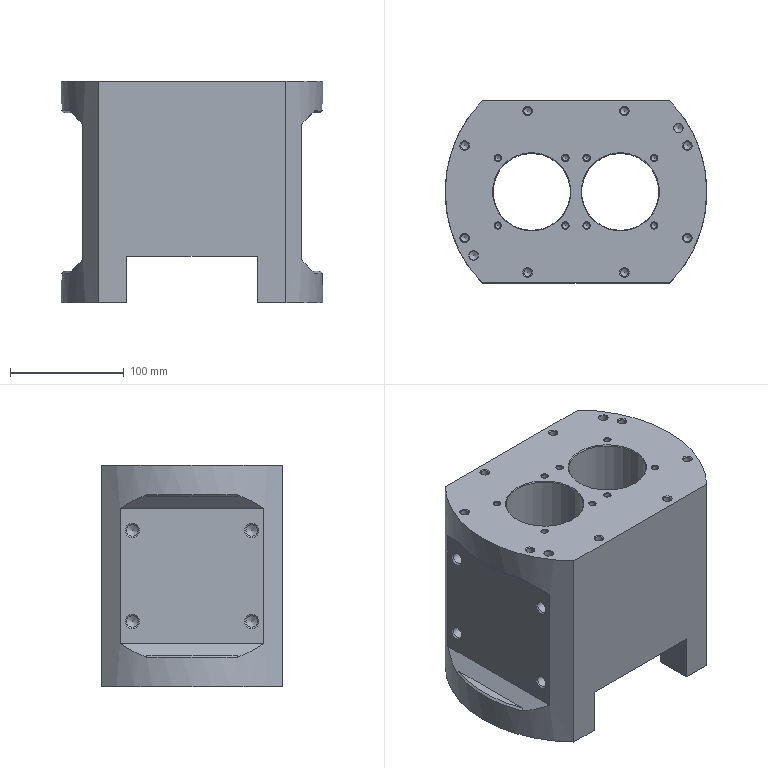NC program | NX | posted with a generic post | part box 230 x 160 x 195 mm
Whole program:
N10 G17 G21 G94 G90
(FLOOR_WALL_COPY_1 , TOOL : D50)
N12 T02 M6
N14 G54
N16 G17 G0 G90 X46.956 Y-107.497 B0. C0. S1200 M3
N18 G43 Z30. H2
N20 Z2.651
N22 G94 G1 Z-0.349 F1000.
N24 X43.956
N26 X-43.956 F2000.
N28 Y-68.498
N30 X43.956
N32 Y-29.498
N34 X-43.956
N36 Y9.501
N38 X43.956
N40 Y48.501
N42 X-43.956
N44 Y87.5
N46 X43.956
N48 X46.956
N50 Z2.651
N52 G0 Z30.
N54 X50.654 Y-107.497
N56 Z2.302
N58 G1 Z-0.698 F1000.
N60 X47.654
N62 X-47.654 F2000.
N64 Y-68.498
N66 X47.654
N68 Y-29.498
N70 X-47.654
N72 Y9.501
N74 X47.654
N76 Y48.501
N78 X-47.654
N80 Y87.5
N82 X47.654
N84 X50.654
N86 Z2.302
N88 G0 Z30.
N90 X53.485 Y-107.497
N92 Z1.953
N94 G1 Z-1.047 F1000.
N96 X50.485
N98 X-50.485 F2000.
N100 Y-68.498
N102 X50.485
N104 Y-29.498
N106 X-50.485
N108 Y9.501
N110 X50.485
N112 Y48.501
N114 X-50.485
N116 Y87.5
N118 X50.485
N120 X53.485
N122 Z1.953
N124 G0 Z30.
N126 X55.866 Y-107.497
N128 Z1.604
N130 G1 Z-1.396 F1000.
N132 X52.866
N134 X-52.866 F2000.
N136 Y-68.498
N138 X52.866
N140 Y-29.498
N142 X-52.866
N144 Y9.501
N146 X52.866
N148 Y48.501
N150 X-52.866
N152 Y87.5
N154 X52.866
N156 X55.866
N158 Z1.604
N160 G0 Z30.
N162 X57.959 Y-107.497
N164 Z1.255
N166 G1 Z-1.745 F1000.
N168 X54.959
N170 X-54.959 F2000.
N172 Y-68.498
N174 X54.959
N176 Y-29.498
N178 X-54.959
N180 Y9.501
N182 X54.959
N184 Y48.501
N186 X-54.959
N188 Y87.5
N190 X54.959
N192 X57.959
N194 Z1.255
N196 G0 Z30.
N198 X59.847 Y-107.497
N200 Z0.906
N202 G1 Z-2.094 F1000.
N204 X56.847
N206 X-56.847 F2000.
N208 Y-68.498
N210 X56.847
N212 Y-29.498
N214 X-56.847
N216 Y9.501
N218 X56.847
N220 Y48.501
N222 X-56.847
N224 Y87.5
N226 X56.847
N228 X59.847
N230 Z0.906
N232 G0 Z30.
N234 X61.579 Y-107.497
N236 Z0.557
N238 G1 Z-2.443 F1000.
N240 X58.579
N242 X-58.579 F2000.
N244 Y-68.498
N246 X58.579
N248 Y-29.498
N250 X-58.579
N252 Y9.501
N254 X58.579
N256 Y48.501
N258 X-58.579
N260 Y87.5
N262 X58.579
N264 X61.579
N266 Z0.557
N268 G0 Z30.
N270 X63.188 Y-107.497
N272 Z0.208
N274 G1 Z-2.792 F1000.
N276 X60.188
N278 X-60.188 F2000.
N280 Y-68.498
N282 X60.188
N284 Y-29.498
N286 X-60.188
N288 Y9.501
N290 X60.188
N292 Y48.501
N294 X-60.188
N296 Y87.5
N298 X60.188
N300 X63.188
N302 Z0.208
N304 G0 Z30.
N306 X64.695 Y-107.497
N308 Z-0.141
N310 G1 Z-3.141 F1000.
N312 X61.695
N314 X-61.695 F2000.
N316 Y-68.498
N318 X61.695
N320 Y-29.498
N322 X-61.695
N324 Y9.501
N326 X61.695
N328 Y48.501
N330 X-61.695
N332 Y87.5
N334 X61.695
N336 X64.695
N338 Z-0.141
N340 G0 Z30.
N342 X66.117 Y-107.497
N344 Z-0.49
N346 G1 Z-3.49 F1000.
N348 X63.117
N350 X-63.117 F2000.
N352 Y-68.498
N354 X63.117
N356 Y-29.498
N358 X-63.117
N360 Y9.501
N362 X63.117
N364 Y48.501
N366 X-63.117
N368 Y87.5
N370 X63.117
N372 X66.117
N374 Z-0.49
N376 G0 Z30.
N378 X67.467 Y-107.497
N380 Z-0.839
N382 G1 Z-3.839 F1000.
N384 X64.467
N386 X-64.467 F2000.
N388 Y-68.498
N390 X64.467
N392 Y-29.498
N394 X-64.467
N396 Y9.501
N398 X64.467
N400 Y48.501
N402 X-64.467
N404 Y87.5
N406 X64.467
N408 X67.467
N410 Z-0.839
N412 G0 Z30.
N414 X68.753 Y-107.497
N416 Z-1.188
N418 G1 Z-4.188 F1000.
N420 X65.753
N422 X-65.753 F2000.
N424 Y-68.498
N426 X65.753
N428 Y-29.498
N430 X-65.753
N432 Y9.501
N434 X65.753
N436 Y48.501
N438 X-65.753
N440 Y87.5
N442 X65.753
N444 X68.753
N446 Z-1.188
N448 G0 Z30.
N450 X69.984 Y-107.497
N452 Z-1.537
N454 G1 Z-4.537 F1000.
N456 X66.984
N458 X-66.984 F2000.
N460 Y-68.498
N462 X66.984
N464 Y-29.498
N466 X-66.984
N468 Y9.501
N470 X66.984
N472 Y48.501
N474 X-66.984
N476 Y87.5
N478 X66.984
N480 X69.984
N482 Z-1.537
N484 G0 Z30.
N486 X71.166 Y-107.497
N488 Z-1.886
N490 G1 Z-4.886 F1000.
N492 X68.166
N494 X-68.166 F2000.
N496 Y-68.498
N498 X68.166
N500 Y-29.498
N502 X-68.166
N504 Y9.501
N506 X68.166
N508 Y48.501
N510 X-68.166
N512 Y87.5
N514 X68.166
N516 X71.166
N518 Z-1.886
N520 G0 Z30.
N522 X72.303 Y-107.497
N524 Z-2.235
N526 G1 Z-5.235 F1000.
N528 X69.303
N530 X-69.303 F2000.
N532 Y-68.498
N534 X69.303
N536 Y-29.498
N538 X-69.303
N540 Y9.501
N542 X69.303
N544 Y48.501
N546 X-69.303
N548 Y87.5
N550 X69.303
N552 X72.303
N554 Z-2.235
N556 G0 Z30.
N558 X73.4 Y-107.497
N560 Z-2.584
N562 G1 Z-5.584 F1000.
N564 X70.4
N566 X-70.4 F2000.
N568 Y-68.498
N570 X70.4
N572 Y-29.498
N574 X-70.4
N576 Y9.501
N578 X70.4
N580 Y48.501
N582 X-70.4
N584 Y87.5
N586 X70.4
N588 X73.4
N590 Z-2.584
N592 G0 Z30.
N594 X74.462 Y-107.497
N596 Z-2.933
N598 G1 Z-5.933 F1000.
N600 X71.462
N602 X-71.462 F2000.
N604 Y-68.498
N606 X71.462
N608 Y-29.498
N610 X-71.462
N612 Y9.501
N614 X71.462
N616 Y48.501
N618 X-71.462
N620 Y87.5
N622 X71.462
N624 X74.462
N626 Z-2.933
N628 G0 Z30.
N630 X75.489 Y-107.497
N632 Z-3.282
N634 G1 Z-6.282 F1000.
N636 X72.489
N638 X-72.489 F2000.
N640 Y-68.498
N642 X72.489
N644 Y-29.498
N646 X-72.489
N648 Y9.501
N650 X72.489
N652 Y48.501
N654 X-72.489
N656 Y87.5
N658 X72.489
N660 X75.489
N662 Z-3.282
N664 G0 Z30.
N666 X76.487 Y-107.497
N668 Z-3.631
N670 G1 Z-6.631 F1000.
N672 X73.487
N674 X-73.487 F2000.
N676 Y-68.498
N678 X73.487
N680 Y-29.498
N682 X-73.487
N684 Y9.501
N686 X73.487
N688 Y48.501
N690 X-73.487
N692 Y87.5
N694 X73.487
N696 X76.487
N698 Z-3.631
N700 G0 Z30.
N702 X77.455 Y-107.497
N704 Z-3.98
N706 G1 Z-6.98 F1000.
N708 X74.455
N710 X-74.455 F2000.
N712 Y-68.498
N714 X74.455
N716 Y-29.498
N718 X-74.455
N720 Y9.501
N722 X74.455
N724 Y48.501
N726 X-74.455
N728 Y87.5
N730 X74.455
N732 X77.455
N734 Z-3.98
N736 G0 Z30.
N738 X78.398 Y-107.497
N740 Z-4.329
N742 G1 Z-7.329 F1000.
N744 X75.398
N746 X-75.398 F2000.
N748 Y-68.498
N750 X75.398
N752 Y-29.498
N754 X-75.398
N756 Y9.501
N758 X75.398
N760 Y48.501
N762 X-75.398
N764 Y87.5
N766 X75.398
N768 X78.398
N770 Z-4.329
N772 G0 Z30.
N774 X79.316 Y-107.497
N776 Z-4.678
N778 G1 Z-7.678 F1000.
N780 X76.316
N782 X-76.316 F2000.
N784 Y-68.498
N786 X76.316
N788 Y-29.498
N790 X-76.316
N792 Y9.501
N794 X76.316
N796 Y48.501
N798 X-76.316
N800 Y87.5
N802 X76.316
N804 X79.316
N806 Z-4.678
N808 G0 Z30.
N810 X80.212 Y-107.497
N812 Z-5.027
N814 G1 Z-8.027 F1000.
N816 X77.212
N818 X-77.212 F2000.
N820 Y-68.498
N822 X77.212
N824 Y-29.498
N826 X-77.212
N828 Y9.501
N830 X77.212
N832 Y48.501
N834 X-77.212
N836 Y87.5
N838 X77.212
N840 X80.212
N842 Z-5.027
N844 G0 Z30.
N846 X81.086 Y-107.497
N848 Z-5.376
N850 G1 Z-8.376 F1000.
N852 X78.086
N854 X-78.086 F2000.
N856 Y-68.498
N858 X78.086
N860 Y-29.498
N862 X-78.086
N864 Y9.501
N866 X78.086
N868 Y48.501
N870 X-78.086
N872 Y87.5
N874 X78.086
N876 X81.086
N878 Z-5.376
N880 G0 Z30.
N882 X81.939 Y-107.497
N884 Z-5.725
N886 G1 Z-8.725 F1000.
N888 X78.939
N890 X-78.939 F2000.
N892 Y-68.498
N894 X78.939
N896 Y-29.498
N898 X-78.939
N900 Y9.501
N902 X78.939
N904 Y48.501
N906 X-78.939
N908 Y87.5
N910 X78.939
N912 X81.939
N914 Z-5.725
N916 G0 Z30.
N918 X82.774 Y-107.497
N920 Z-6.074
N922 G1 Z-9.074 F1000.
N924 X79.774
N926 X-79.774 F2000.
N928 Y-68.498
N930 X79.774
N932 Y-29.498
N934 X-79.774
N936 Y9.501
N938 X79.774
N940 Y48.501
N942 X-79.774
N944 Y87.5
N946 X79.774
N948 X82.774
N950 Z-6.074
N952 G0 Z30.
N954 X83.591 Y-107.497
N956 Z-6.423
N958 G1 Z-9.423 F1000.
N960 X80.591
N962 X-80.591 F2000.
N964 Y-68.498
N966 X80.591
N968 Y-29.498
N970 X-80.591
N972 Y9.501
N974 X80.591
N976 Y48.501
N978 X-80.591
N980 Y87.5
N982 X80.591
N984 X83.591
N986 Z-6.423
N988 G0 Z30.
N990 X84.391 Y-107.497
N992 Z-6.772
N994 G1 Z-9.772 F1000.
N996 X81.391
N998 X-81.391 F2000.
N1000 Y-68.498
N1002 X81.391
N1004 Y-29.498
N1006 X-81.391
N1008 Y9.501
N1010 X81.391
N1012 Y48.501
N1014 X-81.391
N1016 Y87.5
N1018 X81.391
N1020 X84.391
N1022 Z-6.772
N1024 G0 Z30.
N1026 X85.175 Y-107.497
N1028 Z-7.121
N1030 G1 Z-10.121 F1000.
N1032 X82.175
N1034 X-82.175 F2000.
N1036 Y-68.498
N1038 X82.175
N1040 Y-29.498
N1042 X-82.175
N1044 Y9.501
N1046 X82.175
N1048 Y48.501
N1050 X-82.175
N1052 Y87.5
N1054 X82.175
N1056 X85.175
N1058 Z-7.121
N1060 G0 Z30.
N1062 X85.943 Y-107.497
N1064 Z-7.47
N1066 G1 Z-10.47 F1000.
N1068 X82.943
N1070 X-82.943 F2000.
N1072 Y-68.498
N1074 X82.943
N1076 Y-29.498
N1078 X-82.943
N1080 Y9.501
N1082 X82.943
N1084 Y48.501
N1086 X-82.943
N1088 Y87.5
N1090 X82.943
N1092 X85.943
N1094 Z-7.47
N1096 G0 Z30.
N1098 X86.697 Y-107.497
N1100 Z-7.819
N1102 G1 Z-10.819 F1000.
N1104 X83.697
N1106 X-83.697 F2000.
N1108 Y-68.498
N1110 X83.697
N1112 Y-29.498
N1114 X-83.697
N1116 Y9.501
N1118 X83.697
N1120 Y48.501
N1122 X-83.697
N1124 Y87.5
N1126 X83.697
N1128 X86.697
N1130 Z-7.819
N1132 G0 Z30.
N1134 X87.436 Y-107.497
N1136 Z-8.168
N1138 G1 Z-11.168 F1000.
N1140 X84.436
N1142 X-84.436 F2000.
N1144 Y-68.498
N1146 X84.436
N1148 Y-29.498
N1150 X-84.436
N1152 Y9.501
N1154 X84.436
N1156 Y48.501
N1158 X-84.436
N1160 Y87.5
N1162 X84.436
N1164 X87.436
N1166 Z-8.168
N1168 G0 Z30.
N1170 X88.163 Y-107.497
N1172 Z-8.517
N1174 G1 Z-11.517 F1000.
N1176 X85.163
N1178 X-85.163 F2000.
N1180 Y-68.498
N1182 X85.163
N1184 Y-29.498
N1186 X-85.163
N1188 Y9.501
N1190 X85.163
N1192 Y48.501
N1194 X-85.163
N1196 Y87.5
N1198 X85.163
N1200 X88.163
N1202 Z-8.517
N1204 G0 Z30.
N1206 X88.877 Y-107.497
N1208 Z-8.866
N1210 G1 Z-11.866 F1000.
N1212 X85.877
N1214 X-85.877 F2000.
N1216 Y-68.498
N1218 X85.877
N1220 Y-29.498
N1222 X-85.877
N1224 Y9.501
N1226 X85.877
N1228 Y48.501
N1230 X-85.877
N1232 Y87.5
N1234 X85.877
N1236 X88.877
N1238 Z-8.866
N1240 G0 Z30.
N1242 X89.578 Y-107.497
N1244 Z-9.215
N1246 G1 Z-12.215 F1000.
N1248 X86.578
N1250 X-86.578 F2000.
N1252 Y-68.498
N1254 X86.578
N1256 Y-29.498
N1258 X-86.578
N1260 Y9.501
N1262 X86.578
N1264 Y48.501
N1266 X-86.578
N1268 Y87.5
N1270 X86.578
N1272 X89.578
N1274 Z-9.215
N1276 G0 Z30.
N1278 X90.268 Y-107.497
N1280 Z-9.564
N1282 G1 Z-12.564 F1000.
N1284 X87.268
N1286 X-87.268 F2000.
N1288 Y-68.498
N1290 X87.268
N1292 Y-29.498
N1294 X-87.268
N1296 Y9.501
N1298 X87.268
N1300 Y48.501
N1302 X-87.268
N1304 Y87.5
N1306 X87.268
N1308 X90.268
N1310 Z-9.564
N1312 G0 Z30.
N1314 X90.946 Y-107.497
N1316 Z-9.913
N1318 G1 Z-12.913 F1000.
N1320 X87.946
N1322 X-87.946 F2000.
N1324 Y-68.498
N1326 X87.946
N1328 Y-29.498
N1330 X-87.946
N1332 Y9.501
N1334 X87.946
N1336 Y48.501
N1338 X-87.946
N1340 Y87.5
N1342 X87.946
N1344 X90.946
N1346 Z-9.913
N1348 G0 Z30.
N1350 X91.614 Y-107.497
N1352 Z-10.262
N1354 G1 Z-13.262 F1000.
N1356 X88.614
N1358 X-88.614 F2000.
N1360 Y-68.498
N1362 X88.614
N1364 Y-29.498
N1366 X-88.614
N1368 Y9.501
N1370 X88.614
N1372 Y48.501
N1374 X-88.614
N1376 Y87.5
N1378 X88.614
N1380 X91.614
N1382 Z-10.262
N1384 G0 Z30.
N1386 X92.271 Y-107.497
N1388 Z-10.611
N1390 G1 Z-13.611 F1000.
N1392 X89.271
N1394 X-89.271 F2000.
N1396 Y-68.498
N1398 X89.271
N1400 Y-29.498
N1402 X-89.271
N1404 Y9.501
N1406 X89.271
N1408 Y48.501
N1410 X-89.271
N1412 Y87.5
N1414 X89.271
N1416 X92.271
N1418 Z-10.611
N1420 G0 Z30.
N1422 X92.918 Y-107.497
N1424 Z-10.96
N1426 G1 Z-13.96 F1000.
N1428 X89.918
N1430 X-89.918 F2000.
N1432 Y-68.498
N1434 X89.918
N1436 Y-29.498
N1438 X-89.918
N1440 Y9.501
N1442 X89.918
N1444 Y48.501
N1446 X-89.918
N1448 Y87.5
N1450 X89.918
N1452 X92.918
N1454 Z-10.96
N1456 G0 Z30.
N1458 X93.555 Y-107.497
N1460 Z-11.309
N1462 G1 Z-14.309 F1000.
N1464 X90.555
N1466 X-90.555 F2000.
N1468 Y-68.498
N1470 X90.555
N1472 Y-29.498
N1474 X-90.555
N1476 Y9.501
N1478 X90.555
N1480 Y48.501
N1482 X-90.555
N1484 Y87.5
N1486 X90.555
N1488 X93.555
N1490 Z-11.309
N1492 G0 Z30.
N1494 X94.183 Y-107.497
N1496 Z-11.658
N1498 G1 Z-14.658 F1000.
N1500 X91.183
N1502 X-91.183 F2000.
N1504 Y-68.498
N1506 X91.183
N1508 Y-29.498
N1510 X-91.183
N1512 Y9.501
N1514 X91.183
N1516 Y48.501
N1518 X-91.183
N1520 Y87.5
N1522 X91.183
N1524 X94.183
N1526 Z-11.658
N1528 G0 Z30.
N1530 X94.802 Y-107.497
N1532 Z-12.007
N1534 G1 Z-15.007 F1000.
N1536 X91.802
N1538 X-91.802 F2000.
N1540 Y-68.498
N1542 X91.802
N1544 Y-29.498
N1546 X-91.802
N1548 Y9.501
N1550 X91.802
N1552 Y48.501
N1554 X-91.802
N1556 Y87.5
N1558 X91.802
N1560 X94.802
N1562 Z-12.007
N1564 G0 Z30.
N1566 X95.412 Y-107.497
N1568 Z-12.356
N1570 G1 Z-15.356 F1000.
N1572 X92.412
N1574 X-92.412 F2000.
N1576 Y-68.498
N1578 X92.412
N1580 Y-29.498
N1582 X-92.412
N1584 Y9.501
N1586 X92.412
N1588 Y48.501
N1590 X-92.412
N1592 Y87.5
N1594 X92.412
N1596 X95.412
N1598 Z-12.356
N1600 G0 Z30.
N1602 X96.013 Y-107.497
N1604 Z-12.705
N1606 G1 Z-15.705 F1000.
N1608 X93.013
N1610 X-93.013 F2000.
N1612 Y-68.498
N1614 X93.013
N1616 Y-29.498
N1618 X-93.013
N1620 Y9.501
N1622 X93.013
N1624 Y48.501
N1626 X-93.013
N1628 Y87.5
N1630 X93.013
N1632 X96.013
N1634 Z-12.705
N1636 G0 Z30.
N1638 X96.606 Y-107.497
N1640 Z-13.054
N1642 G1 Z-16.054 F1000.
N1644 X93.606
N1646 X-93.606 F2000.
N1648 Y-68.498
N1650 X93.606
N1652 Y-29.498
N1654 X-93.606
N1656 Y9.501
N1658 X93.606
N1660 Y48.501
N1662 X-93.606
N1664 Y87.5
N1666 X93.606
N1668 X96.606
N1670 Z-13.054
N1672 G0 Z30.
N1674 X97.192 Y-107.497
N1676 Z-13.403
N1678 G1 Z-16.403 F1000.
N1680 X94.192
N1682 X-94.192 F2000.
N1684 Y-68.498
N1686 X94.192
N1688 Y-29.498
N1690 X-94.192
N1692 Y9.501
N1694 X94.192
N1696 Y48.501
N1698 X-94.192
N1700 Y87.5
N1702 X94.192
N1704 X97.192
N1706 Z-13.403
N1708 G0 Z30.
N1710 X97.769 Y-107.497
N1712 Z-13.752
N1714 G1 Z-16.752 F1000.
N1716 X94.769
N1718 X-94.769 F2000.
N1720 Y-68.498
N1722 X94.769
N1724 Y-29.498
N1726 X-94.769
N1728 Y9.501
N1730 X94.769
N1732 Y48.501
N1734 X-94.769
N1736 Y87.5
N1738 X94.769
N1740 X97.769
N1742 Z-13.752
N1744 G0 Z30.
N1746 X98.339 Y-107.497
N1748 Z-14.101
N1750 G1 Z-17.101 F1000.
N1752 X95.339
N1754 X-95.339 F2000.
N1756 Y-68.498
N1758 X95.339
N1760 Y-29.498
N1762 X-95.339
N1764 Y9.501
N1766 X95.339
N1768 Y48.501
N1770 X-95.339
N1772 Y87.5
N1774 X95.339
N1776 X98.339
N1778 Z-14.101
N1780 G0 Z30.
N1782 X98.902 Y-107.497
N1784 Z-14.45
N1786 G1 Z-17.45 F1000.
N1788 X95.902
N1790 X-95.902 F2000.
N1792 Y-68.498
N1794 X95.902
N1796 Y-29.498
N1798 X-95.902
N1800 Y9.501
N1802 X95.902
N1804 Y48.501
N1806 X-95.902
N1808 Y87.5
N1810 X95.902
N1812 X98.902
N1814 Z-14.45
N1816 G0 Z30.
N1818 X99.457 Y-107.497
N1820 Z-14.799
N1822 G1 Z-17.799 F1000.
N1824 X96.457
N1826 X-96.457 F2000.
N1828 Y-68.498
N1830 X96.457
N1832 Y-29.498
N1834 X-96.457
N1836 Y9.501
N1838 X96.457
N1840 Y48.501
N1842 X-96.457
N1844 Y87.5
N1846 X96.457
N1848 X99.457
N1850 Z-14.799
N1852 G0 Z30.
N1854 X100.006 Y-107.497
N1856 Z-15.148
N1858 G1 Z-18.148 F1000.
N1860 X97.006
N1862 X-97.006 F2000.
N1864 Y-68.498
N1866 X97.006
N1868 Y-29.498
N1870 X-97.006
N1872 Y9.501
N1874 X97.006
N1876 Y48.501
N1878 X-97.006
N1880 Y87.5
N1882 X97.006
N1884 X100.006
N1886 Z-15.148
N1888 G0 Z30.
N1890 X100.548 Y-107.497
N1892 Z-15.497
N1894 G1 Z-18.497 F1000.
N1896 X97.548
N1898 X-97.548 F2000.
N1900 Y-68.498
N1902 X97.548
N1904 Y-29.498
N1906 X-97.548
N1908 Y9.501
N1910 X97.548
N1912 Y48.501
N1914 X-97.548
N1916 Y87.5
N1918 X97.548
N1920 X100.548
N1922 Z-15.497
N1924 G0 Z30.
N1926 X101.083 Y-107.497
N1928 Z-15.846
N1930 G1 Z-18.846 F1000.
N1932 X98.083
N1934 X-98.083 F2000.
N1936 Y-68.498
N1938 X98.083
N1940 Y-29.498
N1942 X-98.083
N1944 Y9.501
N1946 X98.083
N1948 Y48.501
N1950 X-98.083
N1952 Y87.5
N1954 X98.083
N1956 X101.083
N1958 Z-15.846
N1960 G0 Z30.
N1962 X101.612 Y-107.497
N1964 Z-16.195
N1966 G1 Z-19.195 F1000.
N1968 X98.612
N1970 X-98.612 F2000.
N1972 Y-68.498
N1974 X98.612
N1976 Y-29.498
N1978 X-98.612
N1980 Y9.501
N1982 X98.612
N1984 Y48.501
N1986 X-98.612
N1988 Y87.5
N1990 X98.612
N1992 X101.612
N1994 Z-16.195
N1996 G0 Z30.
N1998 X102.134 Y-107.497
N2000 Z-16.544
N2002 G1 Z-19.544 F1000.
N2004 X99.134
N2006 X-99.134 F2000.
N2008 Y-68.498
N2010 X99.134
N2012 Y-29.498
N2014 X-99.134
N2016 Y9.501
N2018 X99.134
N2020 Y48.501
N2022 X-99.134
N2024 Y87.5
N2026 X99.134
N2028 X102.134
N2030 Z-16.544
N2032 G0 Z30.
N2034 X102.65 Y-107.497
N2036 Z-16.893
N2038 G1 Z-19.893 F1000.
N2040 X99.65
N2042 X-99.65 F2000.
N2044 Y-68.498
N2046 X99.65
N2048 Y-29.498
N2050 X-99.65
N2052 Y9.501
N2054 X99.65
N2056 Y48.501
N2058 X-99.65
N2060 Y87.5
N2062 X99.65
N2064 X102.65
N2066 Z-16.893
N2068 G0 Z30.
N2070 X103.161 Y-107.497
N2072 Z-17.242
N2074 G1 Z-20.242 F1000.
N2076 X100.161
N2078 X-100.161 F2000.
N2080 Y-68.498
N2082 X100.161
N2084 Y-29.498
N2086 X-100.161
N2088 Y9.501
N2090 X100.161
N2092 Y48.501
N2094 X-100.161
N2096 Y87.5
N2098 X100.161
N2100 X103.161
N2102 Z-17.242
N2104 G0 Z30.
N2106 X103.666 Y-107.497
N2108 Z-17.591
N2110 G1 Z-20.591 F1000.
N2112 X100.666
N2114 X-100.666 F2000.
N2116 Y-68.498
N2118 X100.666
N2120 Y-29.498
N2122 X-100.666
N2124 Y9.501
N2126 X100.666
N2128 Y48.501
N2130 X-100.666
N2132 Y87.5
N2134 X100.666
N2136 X103.666
N2138 Z-17.591
N2140 G0 Z30.
N2142 X104.164 Y-107.497
N2144 Z-17.94
N2146 G1 Z-20.94 F1000.
N2148 X101.164
N2150 X-101.164 F2000.
N2152 Y-68.498
N2154 X101.164
N2156 Y-29.498
N2158 X-101.164
N2160 Y9.501
N2162 X101.164
N2164 Y48.501
N2166 X-101.164
N2168 Y87.5
N2170 X101.164
N2172 X104.164
N2174 Z-17.94
N2176 G0 Z30.
N2178 X104.658 Y-107.497
N2180 Z-18.289
N2182 G1 Z-21.289 F1000.
N2184 X101.658
N2186 X-101.658 F2000.
N2188 Y-68.498
N2190 X101.658
N2192 Y-29.498
N2194 X-101.658
N2196 Y9.501
N2198 X101.658
N2200 Y48.501
N2202 X-101.658
N2204 Y87.5
N2206 X101.658
N2208 X104.658
N2210 Z-18.289
N2212 G0 Z30.
N2214 X105.146 Y-107.497
N2216 Z-18.638
N2218 G1 Z-21.638 F1000.
N2220 X102.146
N2222 X-102.146 F2000.
N2224 Y-68.498
N2226 X102.146
N2228 Y-29.498
N2230 X-102.146
N2232 Y9.501
N2234 X102.146
N2236 Y48.501
N2238 X-102.146
N2240 Y87.5
N2242 X102.146
N2244 X105.146
N2246 Z-18.638
N2248 G0 Z30.
N2250 X105.628 Y-107.497
N2252 Z-18.987
N2254 G1 Z-21.987 F1000.
N2256 X102.628
N2258 X-102.628 F2000.
N2260 Y-68.498
N2262 X102.628
N2264 Y-29.498
N2266 X-102.628
N2268 Y9.501
N2270 X102.628
N2272 Y48.501
N2274 X-102.628
N2276 Y87.5
N2278 X102.628
N2280 X105.628
N2282 Z-18.987
N2284 G0 Z30.
N2286 X106.106 Y-107.497
N2288 Z-19.336
N2290 G1 Z-22.336 F1000.
N2292 X103.106
N2294 X-103.106 F2000.
N2296 Y-68.498
N2298 X103.106
N2300 Y-29.498
N2302 X-103.106
N2304 Y9.501
N2306 X103.106
N2308 Y48.501
N2310 X-103.106
N2312 Y87.5
N2314 X103.106
N2316 X106.106
N2318 Z-19.336
N2320 G0 Z30.
N2322 X106.578 Y-107.497
N2324 Z-19.685
N2326 G1 Z-22.685 F1000.
N2328 X103.578
N2330 X-103.578 F2000.
N2332 Y-68.498
N2334 X103.578
N2336 Y-29.498
N2338 X-103.578
N2340 Y9.501
N2342 X103.578
N2344 Y48.501
N2346 X-103.578
N2348 Y87.5
N2350 X103.578
N2352 X106.578
N2354 Z-19.685
N2356 G0 Z30.
N2358 X107.045 Y-107.497
N2360 Z-20.034
N2362 G1 Z-23.034 F1000.
N2364 X104.045
N2366 X-104.045 F2000.
N2368 Y-68.498
N2370 X104.045
N2372 Y-29.498
N2374 X-104.045
N2376 Y9.501
N2378 X104.045
N2380 Y48.501
N2382 X-104.045
N2384 Y87.5
N2386 X104.045
N2388 X107.045
N2390 Z-20.034
N2392 G0 Z30.
N2394 X107.508 Y-107.497
N2396 Z-20.383
N2398 G1 Z-23.383 F1000.
N2400 X104.508
N2402 X-104.508 F2000.
N2404 Y-68.498
N2406 X104.508
N2408 Y-29.498
N2410 X-104.508
N2412 Y9.501
N2414 X104.508
N2416 Y48.501
N2418 X-104.508
N2420 Y87.5
N2422 X104.508
N2424 X107.508
N2426 Z-20.383
N2428 G0 Z30.
N2430 X107.965 Y-107.497
N2432 Z-20.732
N2434 G1 Z-23.732 F1000.
N2436 X104.965
N2438 X-104.965 F2000.
N2440 Y-68.498
N2442 X104.965
N2444 Y-29.498
N2446 X-104.965
N2448 Y9.501
N2450 X104.965
N2452 Y48.501
N2454 X-104.965
N2456 Y87.5
N2458 X104.965
N2460 X107.965
N2462 Z-20.732
N2464 G0 Z30.
N2466 X108.418 Y-107.497
N2468 Z-21.081
N2470 G1 Z-24.081 F1000.
N2472 X105.418
N2474 X-105.418 F2000.
N2476 Y-68.498
N2478 X105.418
N2480 Y-29.498
N2482 X-105.418
N2484 Y9.501
N2486 X105.418
N2488 Y48.501
N2490 X-105.418
N2492 Y87.5
N2494 X105.418
N2496 X108.418
N2498 Z-21.081
N2500 G0 Z30.
N2502 X108.867 Y-107.497
N2504 Z-21.43
N2506 G1 Z-24.43 F1000.
N2508 X105.867
N2510 X-105.867 F2000.
N2512 Y-68.498
N2514 X105.867
N2516 Y-29.498
N2518 X-105.867
N2520 Y9.501
N2522 X105.867
N2524 Y48.501
N2526 X-105.867
N2528 Y87.5
N2530 X105.867
N2532 X108.867
N2534 Z-21.43
N2536 G0 Z30.
N2538 X109.31 Y-107.497
N2540 Z-21.779
N2542 G1 Z-24.779 F1000.
N2544 X106.31
N2546 X-106.31 F2000.
N2548 Y-68.498
N2550 X106.31
N2552 Y-29.498
N2554 X-106.31
N2556 Y9.501
N2558 X106.31
N2560 Y48.501
N2562 X-106.31
N2564 Y87.5
N2566 X106.31
N2568 X109.31
N2570 Z-21.779
N2572 G0 Z30.
N2574 X109.75 Y-107.497
N2576 Z-22.128
N2578 G1 Z-25.128 F1000.
N2580 X106.75
N2582 X-106.75 F2000.
N2584 Y-68.498
N2586 X106.75
N2588 Y-29.498
N2590 X-106.75
N2592 Y9.501
N2594 X106.75
N2596 Y48.501
N2598 X-106.75
N2600 Y87.5
N2602 X106.75
N2604 X109.75
N2606 Z-22.128
N2608 G0 Z30.
N2610 X110.185 Y-107.497
N2612 Z-22.477
N2614 G1 Z-25.477 F1000.
N2616 X107.185
N2618 X-107.185 F2000.
N2620 Y-68.498
N2622 X107.185
N2624 Y-29.498
N2626 X-107.185
N2628 Y9.501
N2630 X107.185
N2632 Y48.501
N2634 X-107.185
N2636 Y87.5
N2638 X107.185
N2640 X110.185
N2642 Z-22.477
N2644 G0 Z30.
N2646 X110.616 Y-107.497
N2648 Z-22.826
N2650 G1 Z-25.826 F1000.
N2652 X107.616
N2654 X-107.616 F2000.
N2656 Y-68.498
N2658 X107.616
N2660 Y-29.498
N2662 X-107.616
N2664 Y9.501
N2666 X107.616
N2668 Y48.501
N2670 X-107.616
N2672 Y87.5
N2674 X107.616
N2676 X110.616
N2678 Z-22.826
N2680 G0 Z30.
N2682 X111.042 Y-107.497
N2684 Z-23.175
N2686 G1 Z-26.175 F1000.
N2688 X108.042
N2690 X-108.042 F2000.
N2692 Y-68.498
N2694 X108.042
N2696 Y-29.498
N2698 X-108.042
N2700 Y9.501
N2702 X108.042
N2704 Y48.501
N2706 X-108.042
N2708 Y87.5
N2710 X108.042
N2712 X111.042
N2714 Z-23.175
N2716 G0 Z30.
N2718 X111.464 Y-107.497
N2720 Z-23.524
N2722 G1 Z-26.524 F1000.
N2724 X108.464
N2726 X-108.464 F2000.
N2728 Y-68.498
N2730 X108.464
N2732 Y-29.498
N2734 X-108.464
N2736 Y9.501
N2738 X108.464
N2740 Y48.501
N2742 X-108.464
N2744 Y87.5
N2746 X108.464
N2748 X111.464
N2750 Z-23.524
N2752 G0 Z30.
N2754 X111.883 Y-107.497
N2756 Z-23.873
N2758 G1 Z-26.873 F1000.
N2760 X108.883
N2762 X-108.883 F2000.
N2764 Y-68.498
N2766 X108.883
N2768 Y-29.498
N2770 X-108.883
N2772 Y9.501
N2774 X108.883
N2776 Y48.501
N2778 X-108.883
N2780 Y87.5
N2782 X108.883
N2784 X111.883
N2786 Z-23.873
N2788 G0 Z30.
N2790 X112.297 Y-107.497
N2792 Z-24.222
N2794 G1 Z-27.222 F1000.
N2796 X109.297
N2798 X-109.297 F2000.
N2800 Y-68.498
N2802 X109.297
N2804 Y-29.498
N2806 X-109.297
N2808 Y9.501
N2810 X109.297
N2812 Y48.501
N2814 X-109.297
N2816 Y87.5
N2818 X109.297
N2820 X112.297
N2822 Z-24.222
N2824 G0 Z30.
N2826 X112.707 Y-107.497
N2828 Z-24.571
N2830 G1 Z-27.571 F1000.
N2832 X109.707
N2834 X-109.707 F2000.
N2836 Y-68.498
N2838 X109.707
N2840 Y-29.498
N2842 X-109.707
N2844 Y9.501
N2846 X109.707
N2848 Y48.501
N2850 X-109.707
N2852 Y87.5
N2854 X109.707
N2856 X112.707
N2858 Z-24.571
N2860 G0 Z30.
N2862 X113.114 Y-107.497
N2864 Z-24.92
N2866 G1 Z-27.92 F1000.
N2868 X110.114
N2870 X-110.114 F2000.
N2872 Y-68.498
N2874 X110.114
N2876 Y-29.498
N2878 X-110.114
N2880 Y9.501
N2882 X110.114
N2884 Y48.501
N2886 X-110.114
N2888 Y87.5
N2890 X110.114
N2892 X113.114
N2894 Z-24.92
N2896 G0 Z30.
N2898 X113.517 Y-107.497
N2900 Z-25.269
N2902 G1 Z-28.269 F1000.
N2904 X110.517
N2906 X-110.517 F2000.
N2908 Y-68.498
N2910 X110.517
N2912 Y-29.498
N2914 X-110.517
N2916 Y9.501
N2918 X110.517
N2920 Y48.501
N2922 X-110.517
N2924 Y87.5
N2926 X110.517
N2928 X113.517
N2930 Z-25.269
N2932 G0 Z30.
N2934 X113.915 Y-107.497
N2936 Z-25.618
N2938 G1 Z-28.618 F1000.
N2940 X110.915
N2942 X-110.915 F2000.
N2944 Y-68.498
N2946 X110.915
N2948 Y-29.498
N2950 X-110.915
N2952 Y9.501
N2954 X110.915
N2956 Y48.501
N2958 X-110.915
N2960 Y87.5
N2962 X110.915
N2964 X113.915
N2966 Z-25.618
N2968 G0 Z30.
N2970 X114.311 Y-107.497
N2972 Z-25.967
N2974 G1 Z-28.967 F1000.
N2976 X111.311
N2978 X-111.311 F2000.
N2980 Y-68.498
N2982 X111.311
N2984 Y-29.498
N2986 X-111.311
N2988 Y9.501
N2990 X111.311
N2992 Y48.501
N2994 X-111.311
N2996 Y87.5
N2998 X111.311
N3000 X114.311
N3002 Z-25.967
N3004 G0 Z30.
N3006 X114.702 Y-107.497
N3008 Z-26.316
N3010 G1 Z-29.316 F1000.
N3012 X111.702
N3014 X-111.702 F2000.
N3016 Y-68.498
N3018 X111.702
N3020 Y-29.498
N3022 X-111.702
N3024 Y9.501
N3026 X111.702
N3028 Y48.501
N3030 X-111.702
N3032 Y87.5
N3034 X111.702
N3036 X114.702
N3038 Z-26.316
N3040 G0 Z30.
N3042 X115.091 Y-107.497
N3044 Z-26.665
N3046 G1 Z-29.665 F1000.
N3048 X112.091
N3050 X-112.091 F2000.
N3052 Y-68.498
N3054 X112.091
N3056 Y-29.498
N3058 X-112.091
N3060 Y9.501
N3062 X112.091
N3064 Y48.501
N3066 X-112.091
N3068 Y87.5
N3070 X112.091
N3072 X115.091
N3074 Z-26.665
N3076 G0 Z30.
N3078 X115.475 Y-107.497
N3080 Z-27.014
N3082 G1 Z-30.014 F1000.
N3084 X112.475
N3086 X-112.475 F2000.
N3088 Y-68.498
N3090 X112.475
N3092 Y-29.498
N3094 X-112.475
N3096 Y9.501
N3098 X112.475
N3100 Y48.501
N3102 X-112.475
N3104 Y87.5
N3106 X112.475
N3108 X115.475
N3110 Z-27.014
N3112 G0 Z30.
N3114 X115.856 Y-107.497
N3116 Z-27.363
N3118 G1 Z-30.363 F1000.
N3120 X112.856
N3122 X-112.856 F2000.
N3124 Y-68.498
N3126 X112.856
N3128 Y-29.498
N3130 X-112.856
N3132 Y9.501
N3134 X112.856
N3136 Y48.501
N3138 X-112.856
N3140 Y87.5
N3142 X112.856
N3144 X115.856
N3146 Z-27.363
N3148 G0 Z30.
N3150 X116.234 Y-107.497
N3152 Z-27.712
N3154 G1 Z-30.712 F1000.
N3156 X113.234
N3158 X-113.234 F2000.
N3160 Y-68.498
N3162 X113.234
N3164 Y-29.498
N3166 X-113.234
N3168 Y9.501
N3170 X113.234
N3172 Y48.501
N3174 X-113.234
N3176 Y87.5
N3178 X113.234
N3180 X116.234
N3182 Z-27.712
N3184 G0 Z30.
N3186 X116.608 Y-107.497
N3188 Z-28.061
N3190 G1 Z-31.061 F1000.
N3192 X113.608
N3194 X-113.608 F2000.
N3196 Y-68.498
N3198 X113.608
N3200 Y-29.498
N3202 X-113.608
N3204 Y9.501
N3206 X113.608
N3208 Y48.501
N3210 X-113.608
N3212 Y87.5
N3214 X113.608
N3216 X116.608
N3218 Z-28.061
N3220 G0 Z30.
N3222 X116.979 Y-107.497
N3224 Z-28.41
N3226 G1 Z-31.41 F1000.
N3228 X113.979
N3230 X-113.979 F2000.
N3232 Y-68.498
N3234 X113.979
N3236 Y-29.498
N3238 X-113.979
N3240 Y9.501
N3242 X113.979
N3244 Y48.501
N3246 X-113.979
N3248 Y87.5
N3250 X113.979
N3252 X116.979
N3254 Z-28.41
N3256 G0 Z30.
N3258 X117.347 Y-107.497
N3260 Z-28.759
N3262 G1 Z-31.759 F1000.
N3264 X114.347
N3266 X-114.347 F2000.
N3268 Y-68.498
N3270 X114.347
N3272 Y-29.498
N3274 X-114.347
N3276 Y9.501
N3278 X114.347
N3280 Y48.501
N3282 X-114.347
N3284 Y87.5
N3286 X114.347
N3288 X117.347
N3290 Z-28.759
N3292 G0 Z30.
N3294 X117.711 Y-107.497
N3296 Z-29.108
N3298 G1 Z-32.108 F1000.
N3300 X114.711
N3302 X-114.711 F2000.
N3304 Y-68.498
N3306 X114.711
N3308 Y-29.498
N3310 X-114.711
N3312 Y9.501
N3314 X114.711
N3316 Y48.501
N3318 X-114.711
N3320 Y87.5
N3322 X114.711
N3324 X117.711
N3326 Z-29.108
N3328 G0 Z30.
N3330 X118.073 Y-107.497
N3332 Z-29.457
N3334 G1 Z-32.457 F1000.
N3336 X115.073
N3338 X-115.073 F2000.
N3340 Y-68.498
N3342 X115.073
N3344 Y-29.498
N3346 X-115.073
N3348 Y9.501
N3350 X115.073
N3352 Y48.501
N3354 X-115.073
N3356 Y87.5
N3358 X115.073
N3360 X118.073
N3362 Z-29.457
N3364 G0 Z30.
N3366 X118.431 Y-107.497
N3368 Z-29.806
N3370 G1 Z-32.806 F1000.
N3372 X115.431
N3374 X-115.431 F2000.
N3376 Y-68.498
N3378 X115.431
N3380 Y-29.498
N3382 X-115.431
N3384 Y9.501
N3386 X115.431
N3388 Y48.501
N3390 X-115.431
N3392 Y87.5
N3394 X115.431
N3396 X118.431
N3398 Z-29.806
N3400 G0 Z30.
N3402 X118.786 Y-107.497
N3404 Z-30.155
N3406 G1 Z-33.155 F1000.
N3408 X115.786
N3410 X-115.786 F2000.
N3412 Y-68.498
N3414 X115.786
N3416 Y-29.498
N3418 X-115.786
N3420 Y9.501
N3422 X115.786
N3424 Y48.501
N3426 X-115.786
N3428 Y87.5
N3430 X115.786
N3432 X118.786
N3434 Z-30.155
N3436 G0 Z30.
N3438 X119.138 Y-107.497
N3440 Z-30.504
N3442 G1 Z-33.504 F1000.
N3444 X116.138
N3446 X-116.138 F2000.
N3448 Y-68.498
N3450 X116.138
N3452 Y-29.498
N3454 X-116.138
N3456 Y9.501
N3458 X116.138
N3460 Y48.501
N3462 X-116.138
N3464 Y87.5
N3466 X116.138
N3468 X119.138
N3470 Z-30.504
N3472 G0 Z30.
N3474 X119.487 Y-107.497
N3476 Z-30.853
N3478 G1 Z-33.853 F1000.
N3480 X116.487
N3482 X-116.487 F2000.
N3484 Y-68.498
N3486 X116.487
N3488 Y-29.498
N3490 X-116.487
N3492 Y9.501
N3494 X116.487
N3496 Y48.501
N3498 X-116.487
N3500 Y87.5
N3502 X116.487
N3504 X119.487
N3506 Z-30.853
N3508 G0 Z30.
N3510 X119.833 Y-107.497
N3512 Z-31.202
N3514 G1 Z-34.202 F1000.
N3516 X116.833
N3518 X-116.833 F2000.
N3520 Y-68.498
N3522 X116.833
N3524 Y-29.498
N3526 X-116.833
N3528 Y9.501
N3530 X116.833
N3532 Y48.501
N3534 X-116.833
N3536 Y87.5
N3538 X116.833
N3540 X119.833
N3542 Z-31.202
N3544 G0 Z30.
N3546 X120.176 Y-107.497
N3548 Z-31.551
N3550 G1 Z-34.551 F1000.
N3552 X117.176
N3554 X-117.176 F2000.
N3556 Y-68.498
N3558 X117.176
N3560 Y-29.498
N3562 X-117.176
N3564 Y9.501
N3566 X117.176
N3568 Y48.501
N3570 X-117.176
N3572 Y87.5
N3574 X117.176
N3576 X120.176
N3578 Z-31.551
N3580 G0 Z30.
N3582 X120.517 Y-107.497
N3584 Z-31.9
N3586 G1 Z-34.9 F1000.
N3588 X117.517
N3590 X-117.517 F2000.
N3592 Y-68.498
N3594 X117.517
N3596 Y-29.498
N3598 X-117.517
N3600 Y9.501
N3602 X117.517
N3604 Y48.501
N3606 X-117.517
N3608 Y87.5
N3610 X117.517
N3612 X120.517
N3614 Z-31.9
N3616 G0 Z30.
(FLOOR_WALL_COPY_COPY , TOOL : D50)
N3618 X120.614 Y-107.497 S2500
N3620 Z-32.
N3622 G1 Z-35. F1000.
N3624 X117.614
N3626 X-117.614
N3628 Y-68.498
N3630 X117.614
N3632 Y-29.498
N3634 X-117.614
N3636 Y9.501
N3638 X117.614
N3640 Y48.501
N3642 X-117.614
N3644 Y87.5
N3646 X117.614
N3648 X120.614
N3650 Z-32.
N3652 G0 Z30.
N3654 M5
N3656 M2